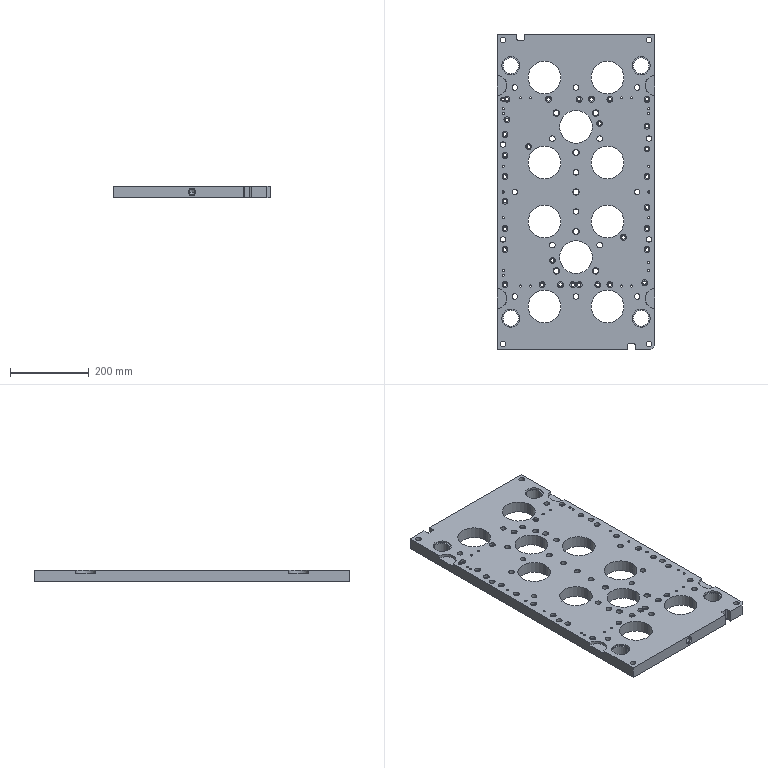Part | Creo | 1 solid | 433 faces | box 400 x 800 x 30 mm | volume 7474722 mm3 | cylinder 320 | plane 77 | cone 36 | commonest cylinder face diameters 9 x62 14 x62 15 x61 5.5 x44 20 x44 83 x20